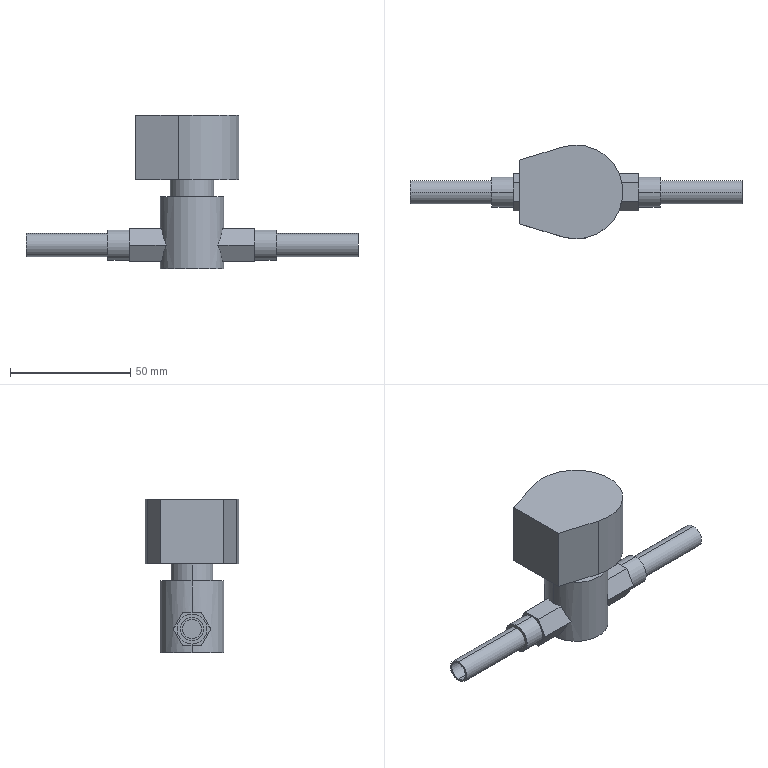Part | STEP file | SEV-603DXF-3-8-cooling solenoid valve | 3 solids | 39 faces | box 138 x 39 x 64 mm | volume 65143 mm3 | plane 26 | cylinder 13 | commonest cylinder face diameters 12.5 x4 8 x2 9.6 x2 18 x2 26.5 x2 39 x1